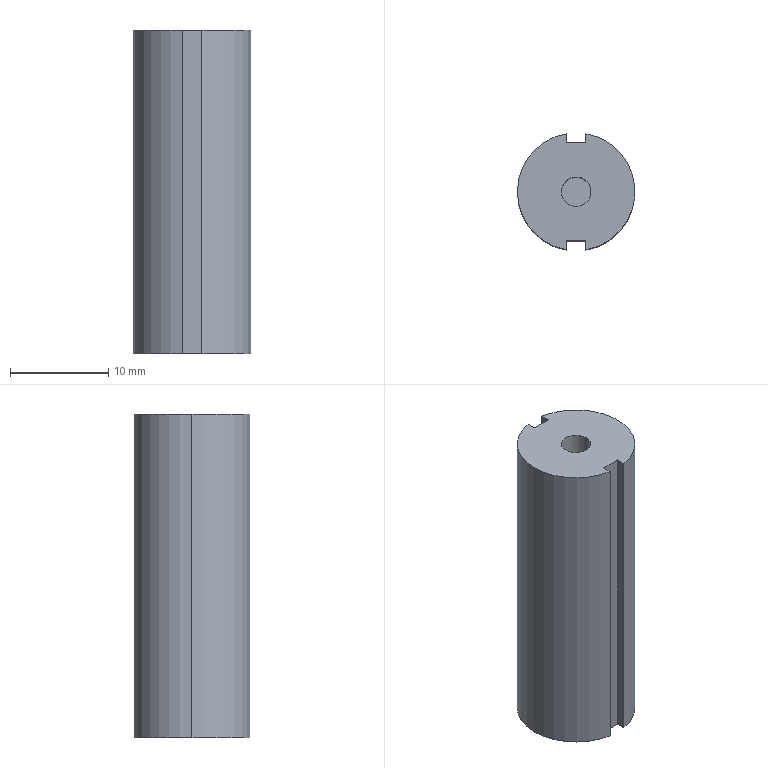Part | SolidWorks | features ICE 5, Extrusion 1, MirrorPattern 1 | 1 solid | 24 faces | box 12 x 11.832 x 33 mm | volume 3415 mm3 | plane 13 | cylinder 11 | commonest cylinder face diameters 12 x3 2 x2 3 x2 6.8 x2 7 x2
STEP:
#1=CARTESIAN_POINT('',(-3.4,0.,0.));
#2=VERTEX_POINT('',#1);
#3=CARTESIAN_POINT('',(3.4,0.,0.));
#4=VERTEX_POINT('',#3);
#5=CARTESIAN_POINT('',(0.,0.,0.));
#6=DIRECTION('',(0.,0.,-1.));
#7=DIRECTION('',(-1.,0.,0.));
#8=AXIS2_PLACEMENT_3D('',#5,#6,#7);
#9=CIRCLE('',#8,3.4);
#10=EDGE_CURVE('',#2,#4,#9,.T.);
#11=ORIENTED_EDGE('',*,*,#10,.F.);
#12=CARTESIAN_POINT('',(-3.4,0.,2.));
#13=VERTEX_POINT('',#12);
#14=CARTESIAN_POINT('',(-3.4,0.,0.));
#15=DIRECTION('',(0.,0.,1.));
#16=VECTOR('',#15,1000.);
#17=LINE('',#14,#16);
#18=EDGE_CURVE('',#2,#13,#17,.T.);
#19=ORIENTED_EDGE('',*,*,#18,.T.);
#20=CARTESIAN_POINT('',(3.4,0.,2.));
#21=VERTEX_POINT('',#20);
#22=CARTESIAN_POINT('',(0.,0.,2.));
#23=DIRECTION('',(0.,0.,-1.));
#24=DIRECTION('',(-1.,0.,0.));
#25=AXIS2_PLACEMENT_3D('',#22,#23,#24);
#26=CIRCLE('',#25,3.4);
#27=EDGE_CURVE('',#13,#21,#26,.T.);
#28=ORIENTED_EDGE('',*,*,#27,.T.);
#29=CARTESIAN_POINT('',(3.4,0.,0.));
#30=DIRECTION('',(0.,0.,1.));
#31=VECTOR('',#30,1000.);
#32=LINE('',#29,#31);
#33=EDGE_CURVE('',#4,#21,#32,.T.);
#34=ORIENTED_EDGE('',*,*,#33,.F.);
#35=EDGE_LOOP('',(#11,#19,#28,#34));
#36=FACE_OUTER_BOUND('',#35,.T.);
#37=CARTESIAN_POINT('',(0.,0.,0.));
#38=DIRECTION('',(0.,0.,1.));
#39=DIRECTION('',(1.,0.,0.));
#40=AXIS2_PLACEMENT_3D('',#37,#38,#39);
#41=CYLINDRICAL_SURFACE('',#40,3.4);
#42=ADVANCED_FACE('',(#36),#41,.T.);
#43=CARTESIAN_POINT('',(3.5,0.,2.));
#44=VERTEX_POINT('',#43);
#45=CARTESIAN_POINT('',(-3.5,0.,2.));
#46=VERTEX_POINT('',#45);
#47=CARTESIAN_POINT('',(0.,0.,2.));
#48=DIRECTION('',(0.,0.,-1.));
#49=DIRECTION('',(-1.,0.,0.));
#50=AXIS2_PLACEMENT_3D('',#47,#48,#49);
#51=CIRCLE('',#50,3.5);
#52=EDGE_CURVE('',#44,#46,#51,.T.);
#53=ORIENTED_EDGE('',*,*,#52,.F.);
#54=CARTESIAN_POINT('',(3.5,0.,0.));
#55=VERTEX_POINT('',#54);
#56=CARTESIAN_POINT('',(3.5,0.,2.));
#57=DIRECTION('',(0.,0.,-1.));
#58=VECTOR('',#57,1000.);
#59=LINE('',#56,#58);
#60=EDGE_CURVE('',#44,#55,#59,.T.);
#61=ORIENTED_EDGE('',*,*,#60,.T.);
#62=CARTESIAN_POINT('',(-3.5,0.,0.));
#63=VERTEX_POINT('',#62);
#64=CARTESIAN_POINT('',(0.,0.,0.));
#65=DIRECTION('',(0.,0.,-1.));
#66=DIRECTION('',(-1.,0.,0.));
#67=AXIS2_PLACEMENT_3D('',#64,#65,#66);
#68=CIRCLE('',#67,3.5);
#69=EDGE_CURVE('',#55,#63,#68,.T.);
#70=ORIENTED_EDGE('',*,*,#69,.T.);
#71=CARTESIAN_POINT('',(-3.5,0.,2.));
#72=DIRECTION('',(0.,0.,-1.));
#73=VECTOR('',#72,1000.);
#74=LINE('',#71,#73);
#75=EDGE_CURVE('',#46,#63,#74,.T.);
#76=ORIENTED_EDGE('',*,*,#75,.F.);
#77=EDGE_LOOP('',(#53,#61,#70,#76));
#78=FACE_OUTER_BOUND('',#77,.T.);
#79=CARTESIAN_POINT('',(0.,0.,2.));
#80=DIRECTION('',(0.,0.,-1.));
#81=DIRECTION('',(-1.,0.,0.));
#82=AXIS2_PLACEMENT_3D('',#79,#80,#81);
#83=CYLINDRICAL_SURFACE('',#82,3.5);
#84=ADVANCED_FACE('',(#78),#83,.F.);
#85=CARTESIAN_POINT('',(0.,-2.,6.));
#86=VERTEX_POINT('',#85);
#87=CARTESIAN_POINT('',(0.,-2.,8.));
#88=VERTEX_POINT('',#87);
#89=CARTESIAN_POINT('',(0.,-2.,7.));
#90=DIRECTION('',(0.,1.,0.));
#91=DIRECTION('',(0.,0.,1.));
#92=AXIS2_PLACEMENT_3D('',#89,#90,#91);
#93=CIRCLE('',#92,1.);
#94=EDGE_CURVE('',#86,#88,#93,.T.);
#95=ORIENTED_EDGE('',*,*,#94,.F.);
#96=CARTESIAN_POINT('',(0.,5.,6.));
#97=VERTEX_POINT('',#96);
#98=CARTESIAN_POINT('',(0.,-2.,6.));
#99=DIRECTION('',(0.,1.,0.));
#100=VECTOR('',#99,1000.);
#101=LINE('',#98,#100);
#102=EDGE_CURVE('',#86,#97,#101,.T.);
#103=ORIENTED_EDGE('',*,*,#102,.T.);
#104=CARTESIAN_POINT('',(-1.,5.,7.));
#105=VERTEX_POINT('',#104);
#106=CARTESIAN_POINT('',(0.,5.,7.));
#107=DIRECTION('',(0.,1.,0.));
#108=DIRECTION('',(0.,0.,1.));
#109=AXIS2_PLACEMENT_3D('',#106,#107,#108);
#110=CIRCLE('',#109,1.);
#111=EDGE_CURVE('',#97,#105,#110,.T.);
#112=ORIENTED_EDGE('',*,*,#111,.T.);
#113=CARTESIAN_POINT('',(0.,5.,8.));
#114=VERTEX_POINT('',#113);
#115=CARTESIAN_POINT('',(0.,5.,7.));
#116=DIRECTION('',(0.,-1.,0.));
#117=DIRECTION('',(0.,0.,-1.));
#118=AXIS2_PLACEMENT_3D('',#115,#116,#117);
#119=CIRCLE('',#118,1.);
#120=EDGE_CURVE('',#114,#105,#119,.T.);
#121=ORIENTED_EDGE('',*,*,#120,.F.);
#122=CARTESIAN_POINT('',(0.,-2.,8.));
#123=DIRECTION('',(0.,1.,0.));
#124=VECTOR('',#123,1000.);
#125=LINE('',#122,#124);
#126=EDGE_CURVE('',#88,#114,#125,.T.);
#127=ORIENTED_EDGE('',*,*,#126,.F.);
#128=EDGE_LOOP('',(#95,#103,#112,#121,#127));
#129=FACE_OUTER_BOUND('',#128,.T.);
#130=CARTESIAN_POINT('',(0.,-2.,7.));
#131=DIRECTION('',(0.,1.,0.));
#132=DIRECTION('',(0.,0.,1.));
#133=AXIS2_PLACEMENT_3D('',#130,#131,#132);
#134=CYLINDRICAL_SURFACE('',#133,1.);
#135=ADVANCED_FACE('',(#129),#134,.F.);
#136=CARTESIAN_POINT('',(-1.5,0.,10.));
#137=VERTEX_POINT('',#136);
#138=CARTESIAN_POINT('',(1.5,0.,10.));
#139=VERTEX_POINT('',#138);
#140=CARTESIAN_POINT('',(0.,0.,10.));
#141=DIRECTION('',(0.,0.,1.));
#142=DIRECTION('',(1.,0.,0.));
#143=AXIS2_PLACEMENT_3D('',#140,#141,#142);
#144=CIRCLE('',#143,1.5);
#145=EDGE_CURVE('',#137,#139,#144,.T.);
#146=ORIENTED_EDGE('',*,*,#145,.F.);
#147=CARTESIAN_POINT('',(-1.5,0.,33.));
#148=VERTEX_POINT('',#147);
#149=CARTESIAN_POINT('',(-1.5,0.,10.));
#150=DIRECTION('',(0.,0.,1.));
#151=VECTOR('',#150,1000.);
#152=LINE('',#149,#151);
#153=EDGE_CURVE('',#137,#148,#152,.T.);
#154=ORIENTED_EDGE('',*,*,#153,.T.);
#155=CARTESIAN_POINT('',(1.5,0.,33.));
#156=VERTEX_POINT('',#155);
#157=CARTESIAN_POINT('',(0.,0.,33.));
#158=DIRECTION('',(0.,0.,1.));
#159=DIRECTION('',(1.,0.,0.));
#160=AXIS2_PLACEMENT_3D('',#157,#158,#159);
#161=CIRCLE('',#160,1.5);
#162=EDGE_CURVE('',#148,#156,#161,.T.);
#163=ORIENTED_EDGE('',*,*,#162,.T.);
#164=CARTESIAN_POINT('',(1.5,0.,10.));
#165=DIRECTION('',(0.,0.,1.));
#166=VECTOR('',#165,1000.);
#167=LINE('',#164,#166);
#168=EDGE_CURVE('',#139,#156,#167,.T.);
#169=ORIENTED_EDGE('',*,*,#168,.F.);
#170=EDGE_LOOP('',(#146,#154,#163,#169));
#171=FACE_OUTER_BOUND('',#170,.T.);
#172=CARTESIAN_POINT('',(0.,0.,10.));
#173=DIRECTION('',(0.,0.,1.));
#174=DIRECTION('',(1.,0.,0.));
#175=AXIS2_PLACEMENT_3D('',#172,#173,#174);
#176=CYLINDRICAL_SURFACE('',#175,1.5);
#177=ADVANCED_FACE('',(#171),#176,.F.);
#178=CARTESIAN_POINT('',(-6.,0.,33.));
#179=VERTEX_POINT('',#178);
#180=CARTESIAN_POINT('',(-1.,-5.916,33.));
#181=VERTEX_POINT('',#180);
#182=CARTESIAN_POINT('',(0.,0.,33.));
#183=DIRECTION('',(0.,0.,1.));
#184=DIRECTION('',(1.,0.,0.));
#185=AXIS2_PLACEMENT_3D('',#182,#183,#184);
#186=CIRCLE('',#185,6.);
#187=EDGE_CURVE('',#179,#181,#186,.T.);
#188=ORIENTED_EDGE('',*,*,#187,.F.);
#189=CARTESIAN_POINT('',(-6.,0.,0.));
#190=VERTEX_POINT('',#189);
#191=CARTESIAN_POINT('',(-6.,0.,33.));
#192=DIRECTION('',(0.,0.,-1.));
#193=VECTOR('',#192,1000.);
#194=LINE('',#191,#193);
#195=EDGE_CURVE('',#179,#190,#194,.T.);
#196=ORIENTED_EDGE('',*,*,#195,.T.);
#197=CARTESIAN_POINT('',(-1.,-5.916,0.));
#198=VERTEX_POINT('',#197);
#199=CARTESIAN_POINT('',(0.,0.,0.));
#200=DIRECTION('',(0.,0.,1.));
#201=DIRECTION('',(1.,0.,0.));
#202=AXIS2_PLACEMENT_3D('',#199,#200,#201);
#203=CIRCLE('',#202,6.);
#204=EDGE_CURVE('',#190,#198,#203,.T.);
#205=ORIENTED_EDGE('',*,*,#204,.T.);
#206=CARTESIAN_POINT('',(-1.,-5.916,33.));
#207=DIRECTION('',(0.,0.,-1.));
#208=VECTOR('',#207,1000.);
#209=LINE('',#206,#208);
#210=EDGE_CURVE('',#181,#198,#209,.T.);
#211=ORIENTED_EDGE('',*,*,#210,.F.);
#212=EDGE_LOOP('',(#188,#196,#205,#211));
#213=FACE_OUTER_BOUND('',#212,.T.);
#214=CARTESIAN_POINT('',(0.,0.,33.));
#215=DIRECTION('',(0.,0.,-1.));
#216=DIRECTION('',(-1.,0.,0.));
#217=AXIS2_PLACEMENT_3D('',#214,#215,#216);
#218=CYLINDRICAL_SURFACE('',#217,6.);
#219=ADVANCED_FACE('',(#213),#218,.T.);
#220=CARTESIAN_POINT('',(1.,5.,7.));
#221=VERTEX_POINT('',#220);
#222=CARTESIAN_POINT('',(1.,5.,33.));
#223=VERTEX_POINT('',#222);
#224=CARTESIAN_POINT('',(1.,5.,0.));
#225=DIRECTION('',(0.,0.,1.));
#226=VECTOR('',#225,1000.);
#227=LINE('',#224,#226);
#228=EDGE_CURVE('',#221,#223,#227,.T.);
#229=ORIENTED_EDGE('',*,*,#228,.F.);
#230=CARTESIAN_POINT('',(0.,5.,7.));
#231=DIRECTION('',(0.,-1.,0.));
#232=DIRECTION('',(0.,0.,-1.));
#233=AXIS2_PLACEMENT_3D('',#230,#231,#232);
#234=CIRCLE('',#233,1.);
#235=EDGE_CURVE('',#221,#114,#234,.T.);
#236=ORIENTED_EDGE('',*,*,#235,.T.);
#237=ORIENTED_EDGE('',*,*,#120,.T.);
#238=CARTESIAN_POINT('',(-1.,5.,33.));
#239=VERTEX_POINT('',#238);
#240=CARTESIAN_POINT('',(-1.,5.,0.));
#241=DIRECTION('',(0.,0.,1.));
#242=VECTOR('',#241,1000.);
#243=LINE('',#240,#242);
#244=EDGE_CURVE('',#105,#239,#243,.T.);
#245=ORIENTED_EDGE('',*,*,#244,.T.);
#246=CARTESIAN_POINT('',(1.,5.,33.));
#247=DIRECTION('',(1.,0.,0.));
#248=VECTOR('',#247,1000.);
#249=LINE('',#246,#248);
#250=EDGE_CURVE('',#239,#223,#249,.T.);
#251=ORIENTED_EDGE('',*,*,#250,.T.);
#252=EDGE_LOOP('',(#229,#236,#237,#245,#251));
#253=FACE_OUTER_BOUND('',#252,.T.);
#254=CARTESIAN_POINT('',(1.,5.,0.));
#255=DIRECTION('',(0.,-1.,0.));
#256=DIRECTION('',(0.,0.,-1.));
#257=AXIS2_PLACEMENT_3D('',#254,#255,#256);
#258=PLANE('',#257);
#259=ADVANCED_FACE('',(#253),#258,.F.);
#260=ORIENTED_EDGE('',*,*,#195,.F.);
#261=CARTESIAN_POINT('',(-1.,5.916,33.));
#262=VERTEX_POINT('',#261);
#263=CARTESIAN_POINT('',(0.,0.,33.));
#264=DIRECTION('',(0.,0.,1.));
#265=DIRECTION('',(1.,0.,0.));
#266=AXIS2_PLACEMENT_3D('',#263,#264,#265);
#267=CIRCLE('',#266,6.);
#268=EDGE_CURVE('',#262,#179,#267,.T.);
#269=ORIENTED_EDGE('',*,*,#268,.F.);
#270=CARTESIAN_POINT('',(-1.,5.916,0.));
#271=VERTEX_POINT('',#270);
#272=CARTESIAN_POINT('',(-1.,5.916,33.));
#273=DIRECTION('',(0.,0.,-1.));
#274=VECTOR('',#273,1000.);
#275=LINE('',#272,#274);
#276=EDGE_CURVE('',#262,#271,#275,.T.);
#277=ORIENTED_EDGE('',*,*,#276,.T.);
#278=CARTESIAN_POINT('',(0.,0.,0.));
#279=DIRECTION('',(0.,0.,1.));
#280=DIRECTION('',(1.,0.,0.));
#281=AXIS2_PLACEMENT_3D('',#278,#279,#280);
#282=CIRCLE('',#281,6.);
#283=EDGE_CURVE('',#271,#190,#282,.T.);
#284=ORIENTED_EDGE('',*,*,#283,.T.);
#285=EDGE_LOOP('',(#260,#269,#277,#284));
#286=FACE_OUTER_BOUND('',#285,.T.);
#287=CARTESIAN_POINT('',(0.,0.,33.));
#288=DIRECTION('',(0.,0.,-1.));
#289=DIRECTION('',(-1.,0.,0.));
#290=AXIS2_PLACEMENT_3D('',#287,#288,#289);
#291=CYLINDRICAL_SURFACE('',#290,6.);
#292=ADVANCED_FACE('',(#286),#291,.T.);
#293=CARTESIAN_POINT('',(1.,-5.916,0.));
#294=VERTEX_POINT('',#293);
#295=CARTESIAN_POINT('',(1.,-5.916,33.));
#296=VERTEX_POINT('',#295);
#297=CARTESIAN_POINT('',(1.,-5.916,33.));
#298=DIRECTION('',(0.,0.,1.));
#299=VECTOR('',#298,1000.);
#300=LINE('',#297,#299);
#301=EDGE_CURVE('',#294,#296,#300,.T.);
#302=ORIENTED_EDGE('',*,*,#301,.F.);
#303=CARTESIAN_POINT('',(1.,5.916,0.));
#304=VERTEX_POINT('',#303);
#305=CARTESIAN_POINT('',(0.,0.,0.));
#306=DIRECTION('',(0.,0.,1.));
#307=DIRECTION('',(1.,0.,0.));
#308=AXIS2_PLACEMENT_3D('',#305,#306,#307);
#309=CIRCLE('',#308,6.);
#310=EDGE_CURVE('',#294,#304,#309,.T.);
#311=ORIENTED_EDGE('',*,*,#310,.T.);
#312=CARTESIAN_POINT('',(1.,5.916,33.));
#313=VERTEX_POINT('',#312);
#314=CARTESIAN_POINT('',(1.,5.916,33.));
#315=DIRECTION('',(0.,0.,1.));
#316=VECTOR('',#315,1000.);
#317=LINE('',#314,#316);
#318=EDGE_CURVE('',#304,#313,#317,.T.);
#319=ORIENTED_EDGE('',*,*,#318,.T.);
#320=CARTESIAN_POINT('',(0.,0.,33.));
#321=DIRECTION('',(0.,0.,1.));
#322=DIRECTION('',(1.,0.,0.));
#323=AXIS2_PLACEMENT_3D('',#320,#321,#322);
#324=CIRCLE('',#323,6.);
#325=EDGE_CURVE('',#296,#313,#324,.T.);
#326=ORIENTED_EDGE('',*,*,#325,.F.);
#327=EDGE_LOOP('',(#302,#311,#319,#326));
#328=FACE_OUTER_BOUND('',#327,.T.);
#329=CARTESIAN_POINT('',(0.,0.,33.));
#330=DIRECTION('',(0.,0.,-1.));
#331=DIRECTION('',(-1.,0.,0.));
#332=AXIS2_PLACEMENT_3D('',#329,#330,#331);
#333=CYLINDRICAL_SURFACE('',#332,6.);
#334=ADVANCED_FACE('',(#328),#333,.T.);
#335=CARTESIAN_POINT('',(0.,0.,33.));
#336=DIRECTION('',(0.,0.,1.));
#337=DIRECTION('',(1.,0.,0.));
#338=AXIS2_PLACEMENT_3D('',#335,#336,#337);
#339=CIRCLE('',#338,1.5);
#340=EDGE_CURVE('',#156,#148,#339,.T.);
#341=ORIENTED_EDGE('',*,*,#340,.F.);
#342=ORIENTED_EDGE('',*,*,#162,.F.);
#343=EDGE_LOOP('',(#341,#342));
#344=FACE_BOUND('',#343,.T.);
#345=ORIENTED_EDGE('',*,*,#268,.T.);
#346=ORIENTED_EDGE('',*,*,#187,.T.);
#347=CARTESIAN_POINT('',(-1.,-5.,33.));
#348=VERTEX_POINT('',#347);
#349=CARTESIAN_POINT('',(-1.,-7.,33.));
#350=DIRECTION('',(0.,1.,0.));
#351=VECTOR('',#350,1000.);
#352=LINE('',#349,#351);
#353=EDGE_CURVE('',#181,#348,#352,.T.);
#354=ORIENTED_EDGE('',*,*,#353,.T.);
#355=CARTESIAN_POINT('',(1.,-5.,33.));
#356=VERTEX_POINT('',#355);
#357=CARTESIAN_POINT('',(1.,-5.,33.));
#358=DIRECTION('',(1.,0.,0.));
#359=VECTOR('',#358,1000.);
#360=LINE('',#357,#359);
#361=EDGE_CURVE('',#348,#356,#360,.T.);
#362=ORIENTED_EDGE('',*,*,#361,.T.);
#363=CARTESIAN_POINT('',(1.,-7.,33.));
#364=DIRECTION('',(0.,-1.,0.));
#365=VECTOR('',#364,1000.);
#366=LINE('',#363,#365);
#367=EDGE_CURVE('',#356,#296,#366,.T.);
#368=ORIENTED_EDGE('',*,*,#367,.T.);
#369=ORIENTED_EDGE('',*,*,#325,.T.);
#370=CARTESIAN_POINT('',(1.,7.,33.));
#371=DIRECTION('',(0.,1.,0.));
#372=VECTOR('',#371,1000.);
#373=LINE('',#370,#372);
#374=EDGE_CURVE('',#223,#313,#373,.T.);
#375=ORIENTED_EDGE('',*,*,#374,.F.);
#376=ORIENTED_EDGE('',*,*,#250,.F.);
#377=CARTESIAN_POINT('',(-1.,7.,33.));
#378=DIRECTION('',(0.,-1.,0.));
#379=VECTOR('',#378,1000.);
#380=LINE('',#377,#379);
#381=EDGE_CURVE('',#262,#239,#380,.T.);
#382=ORIENTED_EDGE('',*,*,#381,.F.);
#383=EDGE_LOOP('',(#345,#346,#354,#362,#368,#369,#375,#376,#382));
#384=FACE_OUTER_BOUND('',#383,.T.);
#385=CARTESIAN_POINT('',(0.,0.,33.));
#386=DIRECTION('',(0.,0.,1.));
#387=DIRECTION('',(1.,0.,0.));
#388=AXIS2_PLACEMENT_3D('',#385,#386,#387);
#389=PLANE('',#388);
#390=ADVANCED_FACE('',(#344,#384),#389,.T.);
#391=CARTESIAN_POINT('',(0.,0.,0.));
#392=DIRECTION('',(0.,0.,-1.));
#393=DIRECTION('',(-1.,0.,0.));
#394=AXIS2_PLACEMENT_3D('',#391,#392,#393);
#395=CIRCLE('',#394,3.5);
#396=EDGE_CURVE('',#63,#55,#395,.T.);
#397=ORIENTED_EDGE('',*,*,#396,.F.);
#398=ORIENTED_EDGE('',*,*,#69,.F.);
#399=EDGE_LOOP('',(#397,#398));
#400=FACE_BOUND('',#399,.T.);
#401=CARTESIAN_POINT('',(-1.,-5.,0.));
#402=VERTEX_POINT('',#401);
#403=CARTESIAN_POINT('',(-1.,0.,0.));
#404=DIRECTION('',(0.,1.,0.));
#405=VECTOR('',#404,1000.);
#406=LINE('',#403,#405);
#407=EDGE_CURVE('',#198,#402,#406,.T.);
#408=ORIENTED_EDGE('',*,*,#407,.F.);
#409=ORIENTED_EDGE('',*,*,#204,.F.);
#410=ORIENTED_EDGE('',*,*,#283,.F.);
#411=CARTESIAN_POINT('',(-1.,5.,0.));
#412=VERTEX_POINT('',#411);
#413=CARTESIAN_POINT('',(-1.,0.,0.));
#414=DIRECTION('',(0.,-1.,0.));
#415=VECTOR('',#414,1000.);
#416=LINE('',#413,#415);
#417=EDGE_CURVE('',#271,#412,#416,.T.);
#418=ORIENTED_EDGE('',*,*,#417,.T.);
#419=CARTESIAN_POINT('',(1.,5.,0.));
#420=VERTEX_POINT('',#419);
#421=CARTESIAN_POINT('',(1.,5.,0.));
#422=DIRECTION('',(1.,0.,0.));
#423=VECTOR('',#422,1000.);
#424=LINE('',#421,#423);
#425=EDGE_CURVE('',#412,#420,#424,.T.);
#426=ORIENTED_EDGE('',*,*,#425,.T.);
#427=CARTESIAN_POINT('',(1.,7.,0.));
#428=DIRECTION('',(0.,1.,0.));
#429=VECTOR('',#428,1000.);
#430=LINE('',#427,#429);
#431=EDGE_CURVE('',#420,#304,#430,.T.);
#432=ORIENTED_EDGE('',*,*,#431,.T.);
#433=ORIENTED_EDGE('',*,*,#310,.F.);
#434=CARTESIAN_POINT('',(1.,-5.,0.));
#435=VERTEX_POINT('',#434);
#436=CARTESIAN_POINT('',(1.,-7.,0.));
#437=DIRECTION('',(0.,-1.,0.));
#438=VECTOR('',#437,1000.);
#439=LINE('',#436,#438);
#440=EDGE_CURVE('',#435,#294,#439,.T.);
#441=ORIENTED_EDGE('',*,*,#440,.F.);
#442=CARTESIAN_POINT('',(1.,-5.,0.));
#443=DIRECTION('',(1.,0.,0.));
#444=VECTOR('',#443,1000.);
#445=LINE('',#442,#444);
#446=EDGE_CURVE('',#402,#435,#445,.T.);
#447=ORIENTED_EDGE('',*,*,#446,.F.);
#448=EDGE_LOOP('',(#408,#409,#410,#418,#426,#432,#433,#441,#447));
#449=FACE_OUTER_BOUND('',#448,.T.);
#450=CARTESIAN_POINT('',(0.,0.,0.));
#451=DIRECTION('',(0.,0.,1.));
#452=DIRECTION('',(1.,0.,0.));
#453=AXIS2_PLACEMENT_3D('',#450,#451,#452);
#454=PLANE('',#453);
#455=ADVANCED_FACE('',(#400,#449),#454,.F.);
#456=ORIENTED_EDGE('',*,*,#381,.T.);
#457=ORIENTED_EDGE('',*,*,#244,.F.);
#458=CARTESIAN_POINT('',(-1.,5.,0.));
#459=DIRECTION('',(0.,0.,1.));
#460=VECTOR('',#459,1000.);
#461=LINE('',#458,#460);
#462=EDGE_CURVE('',#412,#105,#461,.T.);
#463=ORIENTED_EDGE('',*,*,#462,.F.);
#464=ORIENTED_EDGE('',*,*,#417,.F.);
#465=ORIENTED_EDGE('',*,*,#276,.F.);
#466=EDGE_LOOP('',(#456,#457,#463,#464,#465));
#467=FACE_OUTER_BOUND('',#466,.T.);
#468=CARTESIAN_POINT('',(-1.,7.,0.));
#469=DIRECTION('',(-1.,0.,0.));
#470=DIRECTION('',(0.,-1.,0.));
#471=AXIS2_PLACEMENT_3D('',#468,#469,#470);
#472=PLANE('',#471);
#473=ADVANCED_FACE('',(#467),#472,.F.);
#474=ORIENTED_EDGE('',*,*,#431,.F.);
#475=CARTESIAN_POINT('',(1.,5.,0.));
#476=DIRECTION('',(0.,0.,1.));
#477=VECTOR('',#476,1000.);
#478=LINE('',#475,#477);
#479=EDGE_CURVE('',#420,#221,#478,.T.);
#480=ORIENTED_EDGE('',*,*,#479,.T.);
#481=ORIENTED_EDGE('',*,*,#228,.T.);
#482=ORIENTED_EDGE('',*,*,#374,.T.);
#483=ORIENTED_EDGE('',*,*,#318,.F.);
#484=EDGE_LOOP('',(#474,#480,#481,#482,#483));
#485=FACE_OUTER_BOUND('',#484,.T.);
#486=CARTESIAN_POINT('',(1.,7.,0.));
#487=DIRECTION('',(1.,0.,0.));
#488=DIRECTION('',(0.,1.,0.));
#489=AXIS2_PLACEMENT_3D('',#486,#487,#488);
#490=PLANE('',#489);
#491=ADVANCED_FACE('',(#485),#490,.F.);
#492=ORIENTED_EDGE('',*,*,#462,.T.);
#493=ORIENTED_EDGE('',*,*,#111,.F.);
#494=CARTESIAN_POINT('',(0.,5.,7.));
#495=DIRECTION('',(0.,1.,0.));
#496=DIRECTION('',(0.,0.,1.));
#497=AXIS2_PLACEMENT_3D('',#494,#495,#496);
#498=CIRCLE('',#497,1.);
#499=EDGE_CURVE('',#221,#97,#498,.T.);
#500=ORIENTED_EDGE('',*,*,#499,.F.);
#501=ORIENTED_EDGE('',*,*,#479,.F.);
#502=ORIENTED_EDGE('',*,*,#425,.F.);
#503=EDGE_LOOP('',(#492,#493,#500,#501,#502));
#504=FACE_OUTER_BOUND('',#503,.T.);
#505=CARTESIAN_POINT('',(1.,5.,0.));
#506=DIRECTION('',(0.,-1.,0.));
#507=DIRECTION('',(0.,0.,-1.));
#508=AXIS2_PLACEMENT_3D('',#505,#506,#507);
#509=PLANE('',#508);
#510=ADVANCED_FACE('',(#504),#509,.F.);
#511=ORIENTED_EDGE('',*,*,#210,.T.);
#512=ORIENTED_EDGE('',*,*,#407,.T.);
#513=CARTESIAN_POINT('',(-1.,-5.,0.));
#514=DIRECTION('',(0.,0.,1.));
#515=VECTOR('',#514,1000.);
#516=LINE('',#513,#515);
#517=EDGE_CURVE('',#402,#348,#516,.T.);
#518=ORIENTED_EDGE('',*,*,#517,.T.);
#519=ORIENTED_EDGE('',*,*,#353,.F.);
#520=EDGE_LOOP('',(#511,#512,#518,#519));
#521=FACE_OUTER_BOUND('',#520,.T.);
#522=CARTESIAN_POINT('',(-1.,-7.,0.));
#523=DIRECTION('',(1.,0.,0.));
#524=DIRECTION('',(0.,1.,0.));
#525=AXIS2_PLACEMENT_3D('',#522,#523,#524);
#526=PLANE('',#525);
#527=ADVANCED_FACE('',(#521),#526,.T.);
#528=ORIENTED_EDGE('',*,*,#301,.T.);
#529=ORIENTED_EDGE('',*,*,#367,.F.);
#530=CARTESIAN_POINT('',(1.,-5.,0.));
#531=DIRECTION('',(0.,0.,1.));
#532=VECTOR('',#531,1000.);
#533=LINE('',#530,#532);
#534=EDGE_CURVE('',#435,#356,#533,.T.);
#535=ORIENTED_EDGE('',*,*,#534,.F.);
#536=ORIENTED_EDGE('',*,*,#440,.T.);
#537=EDGE_LOOP('',(#528,#529,#535,#536));
#538=FACE_OUTER_BOUND('',#537,.T.);
#539=CARTESIAN_POINT('',(1.,-7.,0.));
#540=DIRECTION('',(-1.,0.,0.));
#541=DIRECTION('',(0.,-1.,0.));
#542=AXIS2_PLACEMENT_3D('',#539,#540,#541);
#543=PLANE('',#542);
#544=ADVANCED_FACE('',(#538),#543,.T.);
#545=ORIENTED_EDGE('',*,*,#361,.F.);
#546=ORIENTED_EDGE('',*,*,#517,.F.);
#547=ORIENTED_EDGE('',*,*,#446,.T.);
#548=ORIENTED_EDGE('',*,*,#534,.T.);
#549=EDGE_LOOP('',(#545,#546,#547,#548));
#550=FACE_OUTER_BOUND('',#549,.T.);
#551=CARTESIAN_POINT('',(1.,-5.,0.));
#552=DIRECTION('',(0.,-1.,0.));
#553=DIRECTION('',(0.,0.,-1.));
#554=AXIS2_PLACEMENT_3D('',#551,#552,#553);
#555=PLANE('',#554);
#556=ADVANCED_FACE('',(#550),#555,.T.);
#557=ORIENTED_EDGE('',*,*,#153,.F.);
#558=CARTESIAN_POINT('',(0.,0.,10.));
#559=DIRECTION('',(0.,0.,1.));
#560=DIRECTION('',(1.,0.,0.));
#561=AXIS2_PLACEMENT_3D('',#558,#559,#560);
#562=CIRCLE('',#561,1.5);
#563=EDGE_CURVE('',#139,#137,#562,.T.);
#564=ORIENTED_EDGE('',*,*,#563,.F.);
#565=ORIENTED_EDGE('',*,*,#168,.T.);
#566=ORIENTED_EDGE('',*,*,#340,.T.);
#567=EDGE_LOOP('',(#557,#564,#565,#566));
#568=FACE_OUTER_BOUND('',#567,.T.);
#569=CARTESIAN_POINT('',(0.,0.,10.));
#570=DIRECTION('',(0.,0.,1.));
#571=DIRECTION('',(1.,0.,0.));
#572=AXIS2_PLACEMENT_3D('',#569,#570,#571);
#573=CYLINDRICAL_SURFACE('',#572,1.5);
#574=ADVANCED_FACE('',(#568),#573,.F.);
#575=ORIENTED_EDGE('',*,*,#563,.T.);
#576=ORIENTED_EDGE('',*,*,#145,.T.);
#577=EDGE_LOOP('',(#575,#576));
#578=FACE_OUTER_BOUND('',#577,.T.);
#579=CARTESIAN_POINT('',(0.,0.,10.));
#580=DIRECTION('',(0.,0.,1.));
#581=DIRECTION('',(1.,0.,0.));
#582=AXIS2_PLACEMENT_3D('',#579,#580,#581);
#583=PLANE('',#582);
#584=ADVANCED_FACE('',(#578),#583,.T.);
#585=ORIENTED_EDGE('',*,*,#102,.F.);
#586=CARTESIAN_POINT('',(0.,-2.,7.));
#587=DIRECTION('',(0.,1.,0.));
#588=DIRECTION('',(0.,0.,1.));
#589=AXIS2_PLACEMENT_3D('',#586,#587,#588);
#590=CIRCLE('',#589,1.);
#591=EDGE_CURVE('',#88,#86,#590,.T.);
#592=ORIENTED_EDGE('',*,*,#591,.F.);
#593=ORIENTED_EDGE('',*,*,#126,.T.);
#594=ORIENTED_EDGE('',*,*,#235,.F.);
#595=ORIENTED_EDGE('',*,*,#499,.T.);
#596=EDGE_LOOP('',(#585,#592,#593,#594,#595));
#597=FACE_OUTER_BOUND('',#596,.T.);
#598=CARTESIAN_POINT('',(0.,-2.,7.));
#599=DIRECTION('',(0.,1.,0.));
#600=DIRECTION('',(0.,0.,1.));
#601=AXIS2_PLACEMENT_3D('',#598,#599,#600);
#602=CYLINDRICAL_SURFACE('',#601,1.);
#603=ADVANCED_FACE('',(#597),#602,.F.);
#604=ORIENTED_EDGE('',*,*,#591,.T.);
#605=ORIENTED_EDGE('',*,*,#94,.T.);
#606=EDGE_LOOP('',(#604,#605));
#607=FACE_OUTER_BOUND('',#606,.T.);
#608=CARTESIAN_POINT('',(0.,-2.,7.));
#609=DIRECTION('',(0.,1.,0.));
#610=DIRECTION('',(0.,0.,1.));
#611=AXIS2_PLACEMENT_3D('',#608,#609,#610);
#612=PLANE('',#611);
#613=ADVANCED_FACE('',(#607),#612,.T.);
#614=ORIENTED_EDGE('',*,*,#60,.F.);
#615=CARTESIAN_POINT('',(0.,0.,2.));
#616=DIRECTION('',(0.,0.,-1.));
#617=DIRECTION('',(-1.,0.,0.));
#618=AXIS2_PLACEMENT_3D('',#615,#616,#617);
#619=CIRCLE('',#618,3.5);
#620=EDGE_CURVE('',#46,#44,#619,.T.);
#621=ORIENTED_EDGE('',*,*,#620,.F.);
#622=ORIENTED_EDGE('',*,*,#75,.T.);
#623=ORIENTED_EDGE('',*,*,#396,.T.);
#624=EDGE_LOOP('',(#614,#621,#622,#623));
#625=FACE_OUTER_BOUND('',#624,.T.);
#626=CARTESIAN_POINT('',(0.,0.,2.));
#627=DIRECTION('',(0.,0.,-1.));
#628=DIRECTION('',(-1.,0.,0.));
#629=AXIS2_PLACEMENT_3D('',#626,#627,#628);
#630=CYLINDRICAL_SURFACE('',#629,3.5);
#631=ADVANCED_FACE('',(#625),#630,.F.);
#632=CARTESIAN_POINT('',(0.,0.,2.));
#633=DIRECTION('',(0.,0.,-1.));
#634=DIRECTION('',(-1.,0.,0.));
#635=AXIS2_PLACEMENT_3D('',#632,#633,#634);
#636=CIRCLE('',#635,3.4);
#637=EDGE_CURVE('',#21,#13,#636,.T.);
#638=ORIENTED_EDGE('',*,*,#637,.F.);
#639=ORIENTED_EDGE('',*,*,#27,.F.);
#640=EDGE_LOOP('',(#638,#639));
#641=FACE_BOUND('',#640,.T.);
#642=ORIENTED_EDGE('',*,*,#620,.T.);
#643=ORIENTED_EDGE('',*,*,#52,.T.);
#644=EDGE_LOOP('',(#642,#643));
#645=FACE_OUTER_BOUND('',#644,.T.);
#646=CARTESIAN_POINT('',(0.,0.,2.));
#647=DIRECTION('',(0.,0.,-1.));
#648=DIRECTION('',(-1.,0.,0.));
#649=AXIS2_PLACEMENT_3D('',#646,#647,#648);
#650=PLANE('',#649);
#651=ADVANCED_FACE('',(#641,#645),#650,.T.);
#652=ORIENTED_EDGE('',*,*,#18,.F.);
#653=CARTESIAN_POINT('',(0.,0.,0.));
#654=DIRECTION('',(0.,0.,-1.));
#655=DIRECTION('',(-1.,0.,0.));
#656=AXIS2_PLACEMENT_3D('',#653,#654,#655);
#657=CIRCLE('',#656,3.4);
#658=EDGE_CURVE('',#4,#2,#657,.T.);
#659=ORIENTED_EDGE('',*,*,#658,.F.);
#660=ORIENTED_EDGE('',*,*,#33,.T.);
#661=ORIENTED_EDGE('',*,*,#637,.T.);
#662=EDGE_LOOP('',(#652,#659,#660,#661));
#663=FACE_OUTER_BOUND('',#662,.T.);
#664=CARTESIAN_POINT('',(0.,0.,0.));
#665=DIRECTION('',(0.,0.,1.));
#666=DIRECTION('',(1.,0.,0.));
#667=AXIS2_PLACEMENT_3D('',#664,#665,#666);
#668=CYLINDRICAL_SURFACE('',#667,3.4);
#669=ADVANCED_FACE('',(#663),#668,.T.);
#670=ORIENTED_EDGE('',*,*,#658,.T.);
#671=ORIENTED_EDGE('',*,*,#10,.T.);
#672=EDGE_LOOP('',(#670,#671));
#673=FACE_OUTER_BOUND('',#672,.T.);
#674=CARTESIAN_POINT('',(0.,0.,0.));
#675=DIRECTION('',(0.,0.,-1.));
#676=DIRECTION('',(-1.,0.,0.));
#677=AXIS2_PLACEMENT_3D('',#674,#675,#676);
#678=PLANE('',#677);
#679=ADVANCED_FACE('',(#673),#678,.T.);
#680=CLOSED_SHELL('',(#42,#84,#135,#177,#219,#259,#292,#334,#390,#455,#473,#491,#510,#527,#544,#556,#574,#584,#603,#613,#631,#651,#669,#679));
#681=MANIFOLD_SOLID_BREP('',#680);
#682=CARTESIAN_POINT('',(0.,0.,0.));
#683=DIRECTION('',(0.,0.,1.));
#684=DIRECTION('',(1.,0.,0.));
#685=AXIS2_PLACEMENT_3D('',#682,#683,#684);
#686=(LENGTH_UNIT()NAMED_UNIT(*)SI_UNIT(.MILLI.,.METRE.));
#687=UNCERTAINTY_MEASURE_WITH_UNIT(LENGTH_MEASURE(0.00001),#686,'','');
#688=(NAMED_UNIT(*)PLANE_ANGLE_UNIT()SI_UNIT($,.RADIAN.));
#689=(NAMED_UNIT(*)SI_UNIT($,.STERADIAN.)SOLID_ANGLE_UNIT());
#690=(GEOMETRIC_REPRESENTATION_CONTEXT(3)GLOBAL_UNCERTAINTY_ASSIGNED_CONTEXT((#687))GLOBAL_UNIT_ASSIGNED_CONTEXT((#686,#688,#689))REPRESENTATION_CONTEXT('',''));
#691=ADVANCED_BREP_SHAPE_REPRESENTATION('',(#681,#685),#690);